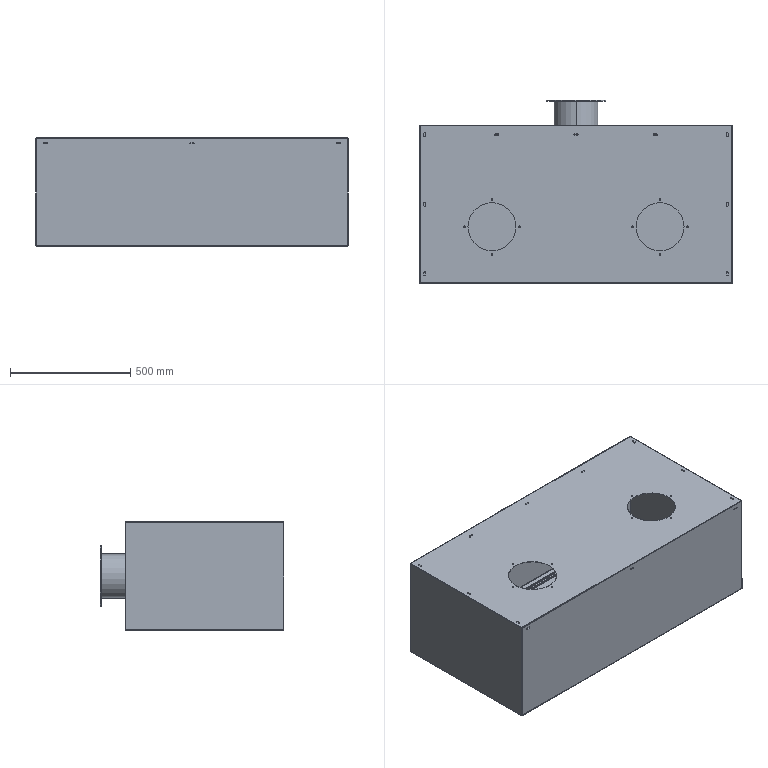Part | SolidWorks | 3 solids | 393 faces | box 1300 x 763 x 450 mm | volume 5569322 mm3 | plane 206 | cylinder 131 | spline 56 | commonest cylinder face diameters 7 x55 1.473 x32 4.473 x32 200 x4 26 x2 180 x2